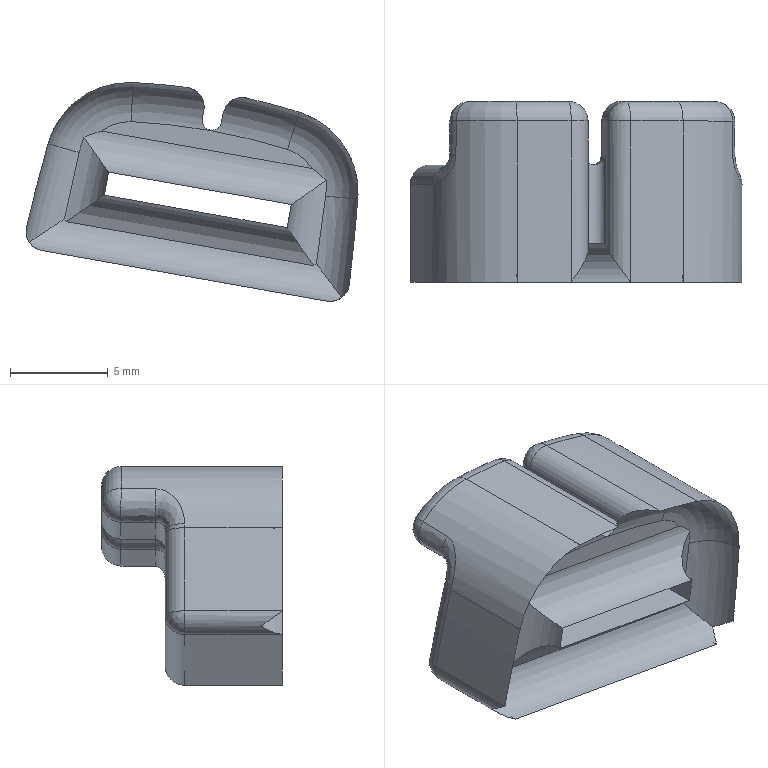Part | SolidWorks | features BaseBody 1 | 1 solid | 70 faces | box 16.984 x 9.25 x 11.199 mm | volume 695.298 mm3 | cylinder 26 | plane 17 | torus 13 | sphere 8 | spline 6 | commonest cylinder face diameters 2 x11 4 x5 1 x4 8.6 x2 67.9 x2 205.1 x2